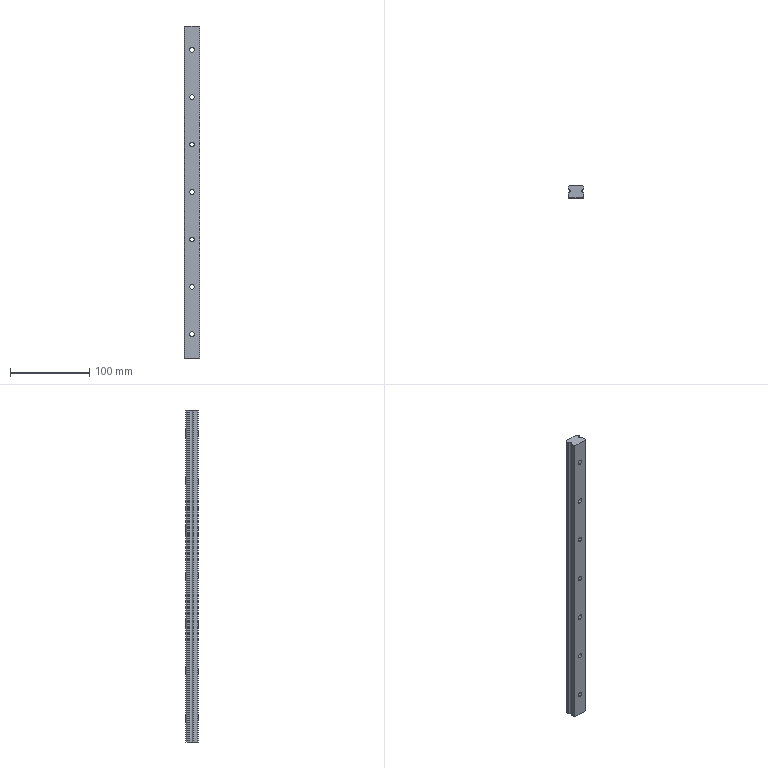Part | SolidWorks | features BaseBody 1 | 1 solid | 51 faces | box 20 x 15.5 x 420 mm | volume 115251 mm3 | cylinder 32 | plane 19 | commonest cylinder face diameters 6 x14 9.5 x14 3 x2 5 x2
STEP:
#1=CARTESIAN_POINT('',(-10.,6.18,-210.));
#2=VERTEX_POINT('',#1);
#3=CARTESIAN_POINT('',(-10.,0.6,-210.));
#4=VERTEX_POINT('',#3);
#5=CARTESIAN_POINT('',(-10.,6.18,-210.));
#6=DIRECTION('',(0.,-1.,0.));
#7=VECTOR('',#6,1000.);
#8=LINE('',#5,#7);
#9=EDGE_CURVE('',#2,#4,#8,.T.);
#10=ORIENTED_EDGE('',*,*,#9,.T.);
#11=CARTESIAN_POINT('',(-10.,0.6,210.));
#12=VERTEX_POINT('',#11);
#13=CARTESIAN_POINT('',(-10.,0.6,210.));
#14=DIRECTION('',(0.,0.,-1.));
#15=VECTOR('',#14,1000.);
#16=LINE('',#13,#15);
#17=EDGE_CURVE('',#12,#4,#16,.T.);
#18=ORIENTED_EDGE('',*,*,#17,.F.);
#19=CARTESIAN_POINT('',(-10.,6.18,210.));
#20=VERTEX_POINT('',#19);
#21=CARTESIAN_POINT('',(-10.,6.18,210.));
#22=DIRECTION('',(0.,-1.,0.));
#23=VECTOR('',#22,1000.);
#24=LINE('',#21,#23);
#25=EDGE_CURVE('',#20,#12,#24,.T.);
#26=ORIENTED_EDGE('',*,*,#25,.F.);
#27=CARTESIAN_POINT('',(-10.,6.18,210.));
#28=DIRECTION('',(0.,0.,-1.));
#29=VECTOR('',#28,1000.);
#30=LINE('',#27,#29);
#31=EDGE_CURVE('',#20,#2,#30,.T.);
#32=ORIENTED_EDGE('',*,*,#31,.T.);
#33=EDGE_LOOP('',(#10,#18,#26,#32));
#34=FACE_OUTER_BOUND('',#33,.T.);
#35=CARTESIAN_POINT('',(-10.,6.18,210.));
#36=DIRECTION('',(1.,0.,0.));
#37=DIRECTION('',(0.,0.,-1.));
#38=AXIS2_PLACEMENT_3D('',#35,#36,#37);
#39=PLANE('',#38);
#40=ADVANCED_FACE('',(#34),#39,.F.);
#41=CARTESIAN_POINT('',(-9.062,10.998,-210.));
#42=VERTEX_POINT('',#41);
#43=CARTESIAN_POINT('',(-10.,8.68,-210.));
#44=DIRECTION('',(0.,0.,1.));
#45=DIRECTION('',(1.,0.,0.));
#46=AXIS2_PLACEMENT_3D('',#43,#44,#45);
#47=CIRCLE('',#46,2.5);
#48=EDGE_CURVE('',#2,#42,#47,.T.);
#49=ORIENTED_EDGE('',*,*,#48,.F.);
#50=ORIENTED_EDGE('',*,*,#31,.F.);
#51=CARTESIAN_POINT('',(-9.062,10.998,210.));
#52=VERTEX_POINT('',#51);
#53=CARTESIAN_POINT('',(-10.,8.68,210.));
#54=DIRECTION('',(0.,0.,1.));
#55=DIRECTION('',(1.,0.,0.));
#56=AXIS2_PLACEMENT_3D('',#53,#54,#55);
#57=CIRCLE('',#56,2.5);
#58=EDGE_CURVE('',#20,#52,#57,.T.);
#59=ORIENTED_EDGE('',*,*,#58,.T.);
#60=CARTESIAN_POINT('',(-9.062,10.998,210.));
#61=DIRECTION('',(0.,0.,-1.));
#62=VECTOR('',#61,1000.);
#63=LINE('',#60,#62);
#64=EDGE_CURVE('',#52,#42,#63,.T.);
#65=ORIENTED_EDGE('',*,*,#64,.T.);
#66=EDGE_LOOP('',(#49,#50,#59,#65));
#67=FACE_OUTER_BOUND('',#66,.T.);
#68=CARTESIAN_POINT('',(-10.,8.68,210.));
#69=DIRECTION('',(0.,0.,-1.));
#70=DIRECTION('',(-0.9816,0.191,0.));
#71=AXIS2_PLACEMENT_3D('',#68,#69,#70);
#72=CYLINDRICAL_SURFACE('',#71,2.5);
#73=ADVANCED_FACE('',(#67),#72,.F.);
#74=CARTESIAN_POINT('',(-10.,12.388,-210.));
#75=VERTEX_POINT('',#74);
#76=CARTESIAN_POINT('',(-8.5,12.388,-210.));
#77=DIRECTION('',(0.,0.,1.));
#78=DIRECTION('',(1.,0.,0.));
#79=AXIS2_PLACEMENT_3D('',#76,#77,#78);
#80=CIRCLE('',#79,1.5);
#81=EDGE_CURVE('',#75,#42,#80,.T.);
#82=ORIENTED_EDGE('',*,*,#81,.T.);
#83=ORIENTED_EDGE('',*,*,#64,.F.);
#84=CARTESIAN_POINT('',(-10.,12.388,210.));
#85=VERTEX_POINT('',#84);
#86=CARTESIAN_POINT('',(-8.5,12.388,210.));
#87=DIRECTION('',(0.,0.,1.));
#88=DIRECTION('',(1.,0.,0.));
#89=AXIS2_PLACEMENT_3D('',#86,#87,#88);
#90=CIRCLE('',#89,1.5);
#91=EDGE_CURVE('',#85,#52,#90,.T.);
#92=ORIENTED_EDGE('',*,*,#91,.F.);
#93=CARTESIAN_POINT('',(-10.,12.388,210.));
#94=DIRECTION('',(0.,0.,-1.));
#95=VECTOR('',#94,1000.);
#96=LINE('',#93,#95);
#97=EDGE_CURVE('',#85,#75,#96,.T.);
#98=ORIENTED_EDGE('',*,*,#97,.T.);
#99=EDGE_LOOP('',(#82,#83,#92,#98));
#100=FACE_OUTER_BOUND('',#99,.T.);
#101=CARTESIAN_POINT('',(-8.5,12.388,210.));
#102=DIRECTION('',(0.,0.,-1.));
#103=DIRECTION('',(0.8292,0.559,0.));
#104=AXIS2_PLACEMENT_3D('',#101,#102,#103);
#105=CYLINDRICAL_SURFACE('',#104,1.5);
#106=ADVANCED_FACE('',(#100),#105,.T.);
#107=CARTESIAN_POINT('',(-10.,14.043,-210.));
#108=VERTEX_POINT('',#107);
#109=CARTESIAN_POINT('',(-10.,14.043,-210.));
#110=DIRECTION('',(0.,-1.,0.));
#111=VECTOR('',#110,1000.);
#112=LINE('',#109,#111);
#113=EDGE_CURVE('',#108,#75,#112,.T.);
#114=ORIENTED_EDGE('',*,*,#113,.T.);
#115=ORIENTED_EDGE('',*,*,#97,.F.);
#116=CARTESIAN_POINT('',(-10.,14.043,210.));
#117=VERTEX_POINT('',#116);
#118=CARTESIAN_POINT('',(-10.,14.043,210.));
#119=DIRECTION('',(0.,-1.,0.));
#120=VECTOR('',#119,1000.);
#121=LINE('',#118,#120);
#122=EDGE_CURVE('',#117,#85,#121,.T.);
#123=ORIENTED_EDGE('',*,*,#122,.F.);
#124=CARTESIAN_POINT('',(-10.,14.043,210.));
#125=DIRECTION('',(0.,0.,-1.));
#126=VECTOR('',#125,1000.);
#127=LINE('',#124,#126);
#128=EDGE_CURVE('',#117,#108,#127,.T.);
#129=ORIENTED_EDGE('',*,*,#128,.T.);
#130=EDGE_LOOP('',(#114,#115,#123,#129));
#131=FACE_OUTER_BOUND('',#130,.T.);
#132=CARTESIAN_POINT('',(-10.,14.043,210.));
#133=DIRECTION('',(1.,0.,0.));
#134=DIRECTION('',(0.,0.,-1.));
#135=AXIS2_PLACEMENT_3D('',#132,#133,#134);
#136=PLANE('',#135);
#137=ADVANCED_FACE('',(#131),#136,.F.);
#138=CARTESIAN_POINT('',(-8.543,15.5,-210.));
#139=VERTEX_POINT('',#138);
#140=CARTESIAN_POINT('',(-8.543,15.5,-210.));
#141=DIRECTION('',(-0.7071,-0.7071,0.));
#142=VECTOR('',#141,1000.);
#143=LINE('',#140,#142);
#144=EDGE_CURVE('',#139,#108,#143,.T.);
#145=ORIENTED_EDGE('',*,*,#144,.T.);
#146=ORIENTED_EDGE('',*,*,#128,.F.);
#147=CARTESIAN_POINT('',(-8.543,15.5,210.));
#148=VERTEX_POINT('',#147);
#149=CARTESIAN_POINT('',(-8.543,15.5,210.));
#150=DIRECTION('',(-0.7071,-0.7071,0.));
#151=VECTOR('',#150,1000.);
#152=LINE('',#149,#151);
#153=EDGE_CURVE('',#148,#117,#152,.T.);
#154=ORIENTED_EDGE('',*,*,#153,.F.);
#155=CARTESIAN_POINT('',(-8.543,15.5,210.));
#156=DIRECTION('',(0.,0.,-1.));
#157=VECTOR('',#156,1000.);
#158=LINE('',#155,#157);
#159=EDGE_CURVE('',#148,#139,#158,.T.);
#160=ORIENTED_EDGE('',*,*,#159,.T.);
#161=EDGE_LOOP('',(#145,#146,#154,#160));
#162=FACE_OUTER_BOUND('',#161,.T.);
#163=CARTESIAN_POINT('',(-8.543,15.5,210.));
#164=DIRECTION('',(0.7071,-0.7071,0.));
#165=DIRECTION('',(0.7071,0.7071,0.));
#166=AXIS2_PLACEMENT_3D('',#163,#164,#165);
#167=PLANE('',#166);
#168=ADVANCED_FACE('',(#162),#167,.F.);
#169=CARTESIAN_POINT('',(0.,15.5,-124.75));
#170=VERTEX_POINT('',#169);
#171=CARTESIAN_POINT('',(0.,15.5,-115.25));
#172=VERTEX_POINT('',#171);
#173=CARTESIAN_POINT('',(0.,15.5,-120.));
#174=DIRECTION('',(0.,-1.,0.));
#175=DIRECTION('',(0.,0.,-1.));
#176=AXIS2_PLACEMENT_3D('',#173,#174,#175);
#177=CIRCLE('',#176,4.75);
#178=EDGE_CURVE('',#170,#172,#177,.T.);
#179=ORIENTED_EDGE('',*,*,#178,.T.);
#180=CARTESIAN_POINT('',(0.,15.5,-120.));
#181=DIRECTION('',(0.,-1.,0.));
#182=DIRECTION('',(0.,0.,-1.));
#183=AXIS2_PLACEMENT_3D('',#180,#181,#182);
#184=CIRCLE('',#183,4.75);
#185=EDGE_CURVE('',#172,#170,#184,.T.);
#186=ORIENTED_EDGE('',*,*,#185,.T.);
#187=EDGE_LOOP('',(#179,#186));
#188=FACE_BOUND('',#187,.T.);
#189=CARTESIAN_POINT('',(0.,15.5,-64.75));
#190=VERTEX_POINT('',#189);
#191=CARTESIAN_POINT('',(0.,15.5,-55.25));
#192=VERTEX_POINT('',#191);
#193=CARTESIAN_POINT('',(0.,15.5,-60.));
#194=DIRECTION('',(0.,-1.,0.));
#195=DIRECTION('',(0.,0.,-1.));
#196=AXIS2_PLACEMENT_3D('',#193,#194,#195);
#197=CIRCLE('',#196,4.75);
#198=EDGE_CURVE('',#190,#192,#197,.T.);
#199=ORIENTED_EDGE('',*,*,#198,.T.);
#200=CARTESIAN_POINT('',(0.,15.5,-60.));
#201=DIRECTION('',(0.,-1.,0.));
#202=DIRECTION('',(0.,0.,-1.));
#203=AXIS2_PLACEMENT_3D('',#200,#201,#202);
#204=CIRCLE('',#203,4.75);
#205=EDGE_CURVE('',#192,#190,#204,.T.);
#206=ORIENTED_EDGE('',*,*,#205,.T.);
#207=EDGE_LOOP('',(#199,#206));
#208=FACE_BOUND('',#207,.T.);
#209=CARTESIAN_POINT('',(0.,15.5,-4.75));
#210=VERTEX_POINT('',#209);
#211=CARTESIAN_POINT('',(0.,15.5,4.75));
#212=VERTEX_POINT('',#211);
#213=CARTESIAN_POINT('',(0.,15.5,0.));
#214=DIRECTION('',(0.,-1.,0.));
#215=DIRECTION('',(0.,0.,-1.));
#216=AXIS2_PLACEMENT_3D('',#213,#214,#215);
#217=CIRCLE('',#216,4.75);
#218=EDGE_CURVE('',#210,#212,#217,.T.);
#219=ORIENTED_EDGE('',*,*,#218,.T.);
#220=CARTESIAN_POINT('',(0.,15.5,0.));
#221=DIRECTION('',(0.,-1.,0.));
#222=DIRECTION('',(0.,0.,-1.));
#223=AXIS2_PLACEMENT_3D('',#220,#221,#222);
#224=CIRCLE('',#223,4.75);
#225=EDGE_CURVE('',#212,#210,#224,.T.);
#226=ORIENTED_EDGE('',*,*,#225,.T.);
#227=EDGE_LOOP('',(#219,#226));
#228=FACE_BOUND('',#227,.T.);
#229=CARTESIAN_POINT('',(0.,15.5,55.25));
#230=VERTEX_POINT('',#229);
#231=CARTESIAN_POINT('',(0.,15.5,64.75));
#232=VERTEX_POINT('',#231);
#233=CARTESIAN_POINT('',(0.,15.5,60.));
#234=DIRECTION('',(0.,-1.,0.));
#235=DIRECTION('',(0.,0.,-1.));
#236=AXIS2_PLACEMENT_3D('',#233,#234,#235);
#237=CIRCLE('',#236,4.75);
#238=EDGE_CURVE('',#230,#232,#237,.T.);
#239=ORIENTED_EDGE('',*,*,#238,.T.);
#240=CARTESIAN_POINT('',(0.,15.5,60.));
#241=DIRECTION('',(0.,-1.,0.));
#242=DIRECTION('',(0.,0.,-1.));
#243=AXIS2_PLACEMENT_3D('',#240,#241,#242);
#244=CIRCLE('',#243,4.75);
#245=EDGE_CURVE('',#232,#230,#244,.T.);
#246=ORIENTED_EDGE('',*,*,#245,.T.);
#247=EDGE_LOOP('',(#239,#246));
#248=FACE_BOUND('',#247,.T.);
#249=CARTESIAN_POINT('',(0.,15.5,115.25));
#250=VERTEX_POINT('',#249);
#251=CARTESIAN_POINT('',(0.,15.5,124.75));
#252=VERTEX_POINT('',#251);
#253=CARTESIAN_POINT('',(0.,15.5,120.));
#254=DIRECTION('',(0.,-1.,0.));
#255=DIRECTION('',(0.,0.,-1.));
#256=AXIS2_PLACEMENT_3D('',#253,#254,#255);
#257=CIRCLE('',#256,4.75);
#258=EDGE_CURVE('',#250,#252,#257,.T.);
#259=ORIENTED_EDGE('',*,*,#258,.T.);
#260=CARTESIAN_POINT('',(0.,15.5,120.));
#261=DIRECTION('',(0.,-1.,0.));
#262=DIRECTION('',(0.,0.,-1.));
#263=AXIS2_PLACEMENT_3D('',#260,#261,#262);
#264=CIRCLE('',#263,4.75);
#265=EDGE_CURVE('',#252,#250,#264,.T.);
#266=ORIENTED_EDGE('',*,*,#265,.T.);
#267=EDGE_LOOP('',(#259,#266));
#268=FACE_BOUND('',#267,.T.);
#269=CARTESIAN_POINT('',(0.,15.5,175.25));
#270=VERTEX_POINT('',#269);
#271=CARTESIAN_POINT('',(0.,15.5,184.75));
#272=VERTEX_POINT('',#271);
#273=CARTESIAN_POINT('',(0.,15.5,180.));
#274=DIRECTION('',(0.,-1.,0.));
#275=DIRECTION('',(0.,0.,-1.));
#276=AXIS2_PLACEMENT_3D('',#273,#274,#275);
#277=CIRCLE('',#276,4.75);
#278=EDGE_CURVE('',#270,#272,#277,.T.);
#279=ORIENTED_EDGE('',*,*,#278,.T.);
#280=CARTESIAN_POINT('',(0.,15.5,180.));
#281=DIRECTION('',(0.,-1.,0.));
#282=DIRECTION('',(0.,0.,-1.));
#283=AXIS2_PLACEMENT_3D('',#280,#281,#282);
#284=CIRCLE('',#283,4.75);
#285=EDGE_CURVE('',#272,#270,#284,.T.);
#286=ORIENTED_EDGE('',*,*,#285,.T.);
#287=EDGE_LOOP('',(#279,#286));
#288=FACE_BOUND('',#287,.T.);
#289=CARTESIAN_POINT('',(0.,15.5,-184.75));
#290=VERTEX_POINT('',#289);
#291=CARTESIAN_POINT('',(0.,15.5,-175.25));
#292=VERTEX_POINT('',#291);
#293=CARTESIAN_POINT('',(0.,15.5,-180.));
#294=DIRECTION('',(0.,-1.,0.));
#295=DIRECTION('',(0.,0.,-1.));
#296=AXIS2_PLACEMENT_3D('',#293,#294,#295);
#297=CIRCLE('',#296,4.75);
#298=EDGE_CURVE('',#290,#292,#297,.T.);
#299=ORIENTED_EDGE('',*,*,#298,.T.);
#300=CARTESIAN_POINT('',(0.,15.5,-180.));
#301=DIRECTION('',(0.,-1.,0.));
#302=DIRECTION('',(0.,0.,-1.));
#303=AXIS2_PLACEMENT_3D('',#300,#301,#302);
#304=CIRCLE('',#303,4.75);
#305=EDGE_CURVE('',#292,#290,#304,.T.);
#306=ORIENTED_EDGE('',*,*,#305,.T.);
#307=EDGE_LOOP('',(#299,#306));
#308=FACE_BOUND('',#307,.T.);
#309=CARTESIAN_POINT('',(8.543,15.5,-210.));
#310=VERTEX_POINT('',#309);
#311=CARTESIAN_POINT('',(8.543,15.5,-210.));
#312=DIRECTION('',(-1.,0.,0.));
#313=VECTOR('',#312,1000.);
#314=LINE('',#311,#313);
#315=EDGE_CURVE('',#310,#139,#314,.T.);
#316=ORIENTED_EDGE('',*,*,#315,.T.);
#317=ORIENTED_EDGE('',*,*,#159,.F.);
#318=CARTESIAN_POINT('',(8.543,15.5,210.));
#319=VERTEX_POINT('',#318);
#320=CARTESIAN_POINT('',(8.543,15.5,210.));
#321=DIRECTION('',(-1.,0.,0.));
#322=VECTOR('',#321,1000.);
#323=LINE('',#320,#322);
#324=EDGE_CURVE('',#319,#148,#323,.T.);
#325=ORIENTED_EDGE('',*,*,#324,.F.);
#326=CARTESIAN_POINT('',(8.543,15.5,210.));
#327=DIRECTION('',(0.,0.,-1.));
#328=VECTOR('',#327,1000.);
#329=LINE('',#326,#328);
#330=EDGE_CURVE('',#319,#310,#329,.T.);
#331=ORIENTED_EDGE('',*,*,#330,.T.);
#332=EDGE_LOOP('',(#316,#317,#325,#331));
#333=FACE_OUTER_BOUND('',#332,.T.);
#334=CARTESIAN_POINT('',(8.543,15.5,210.));
#335=DIRECTION('',(0.,-1.,0.));
#336=DIRECTION('',(0.,0.,-1.));
#337=AXIS2_PLACEMENT_3D('',#334,#335,#336);
#338=PLANE('',#337);
#339=ADVANCED_FACE('',(#188,#208,#228,#248,#268,#288,#308,#333),#338,.F.);
#340=CARTESIAN_POINT('',(10.,14.043,-210.));
#341=VERTEX_POINT('',#340);
#342=CARTESIAN_POINT('',(10.,14.043,-210.));
#343=DIRECTION('',(-0.7071,0.7071,0.));
#344=VECTOR('',#343,1000.);
#345=LINE('',#342,#344);
#346=EDGE_CURVE('',#341,#310,#345,.T.);
#347=ORIENTED_EDGE('',*,*,#346,.T.);
#348=ORIENTED_EDGE('',*,*,#330,.F.);
#349=CARTESIAN_POINT('',(10.,14.043,210.));
#350=VERTEX_POINT('',#349);
#351=CARTESIAN_POINT('',(10.,14.043,210.));
#352=DIRECTION('',(-0.7071,0.7071,0.));
#353=VECTOR('',#352,1000.);
#354=LINE('',#351,#353);
#355=EDGE_CURVE('',#350,#319,#354,.T.);
#356=ORIENTED_EDGE('',*,*,#355,.F.);
#357=CARTESIAN_POINT('',(10.,14.043,210.));
#358=DIRECTION('',(0.,0.,-1.));
#359=VECTOR('',#358,1000.);
#360=LINE('',#357,#359);
#361=EDGE_CURVE('',#350,#341,#360,.T.);
#362=ORIENTED_EDGE('',*,*,#361,.T.);
#363=EDGE_LOOP('',(#347,#348,#356,#362));
#364=FACE_OUTER_BOUND('',#363,.T.);
#365=CARTESIAN_POINT('',(10.,14.043,210.));
#366=DIRECTION('',(-0.7071,-0.7071,0.));
#367=DIRECTION('',(0.7071,-0.7071,0.));
#368=AXIS2_PLACEMENT_3D('',#365,#366,#367);
#369=PLANE('',#368);
#370=ADVANCED_FACE('',(#364),#369,.F.);
#371=CARTESIAN_POINT('',(10.,12.388,-210.));
#372=VERTEX_POINT('',#371);
#373=CARTESIAN_POINT('',(10.,12.388,-210.));
#374=DIRECTION('',(0.,1.,0.));
#375=VECTOR('',#374,1000.);
#376=LINE('',#373,#375);
#377=EDGE_CURVE('',#372,#341,#376,.T.);
#378=ORIENTED_EDGE('',*,*,#377,.T.);
#379=ORIENTED_EDGE('',*,*,#361,.F.);
#380=CARTESIAN_POINT('',(10.,12.388,210.));
#381=VERTEX_POINT('',#380);
#382=CARTESIAN_POINT('',(10.,12.388,210.));
#383=DIRECTION('',(0.,1.,0.));
#384=VECTOR('',#383,1000.);
#385=LINE('',#382,#384);
#386=EDGE_CURVE('',#381,#350,#385,.T.);
#387=ORIENTED_EDGE('',*,*,#386,.F.);
#388=CARTESIAN_POINT('',(10.,12.388,210.));
#389=DIRECTION('',(0.,0.,-1.));
#390=VECTOR('',#389,1000.);
#391=LINE('',#388,#390);
#392=EDGE_CURVE('',#381,#372,#391,.T.);
#393=ORIENTED_EDGE('',*,*,#392,.T.);
#394=EDGE_LOOP('',(#378,#379,#387,#393));
#395=FACE_OUTER_BOUND('',#394,.T.);
#396=CARTESIAN_POINT('',(10.,12.388,210.));
#397=DIRECTION('',(-1.,0.,0.));
#398=DIRECTION('',(0.,0.,1.));
#399=AXIS2_PLACEMENT_3D('',#396,#397,#398);
#400=PLANE('',#399);
#401=ADVANCED_FACE('',(#395),#400,.F.);
#402=CARTESIAN_POINT('',(9.062,10.998,-210.));
#403=VERTEX_POINT('',#402);
#404=CARTESIAN_POINT('',(8.5,12.388,-210.));
#405=DIRECTION('',(0.,0.,1.));
#406=DIRECTION('',(1.,0.,0.));
#407=AXIS2_PLACEMENT_3D('',#404,#405,#406);
#408=CIRCLE('',#407,1.5);
#409=EDGE_CURVE('',#403,#372,#408,.T.);
#410=ORIENTED_EDGE('',*,*,#409,.T.);
#411=ORIENTED_EDGE('',*,*,#392,.F.);
#412=CARTESIAN_POINT('',(9.062,10.998,210.));
#413=VERTEX_POINT('',#412);
#414=CARTESIAN_POINT('',(8.5,12.388,210.));
#415=DIRECTION('',(0.,0.,1.));
#416=DIRECTION('',(1.,0.,0.));
#417=AXIS2_PLACEMENT_3D('',#414,#415,#416);
#418=CIRCLE('',#417,1.5);
#419=EDGE_CURVE('',#413,#381,#418,.T.);
#420=ORIENTED_EDGE('',*,*,#419,.F.);
#421=CARTESIAN_POINT('',(9.062,10.998,210.));
#422=DIRECTION('',(0.,0.,-1.));
#423=VECTOR('',#422,1000.);
#424=LINE('',#421,#423);
#425=EDGE_CURVE('',#413,#403,#424,.T.);
#426=ORIENTED_EDGE('',*,*,#425,.T.);
#427=EDGE_LOOP('',(#410,#411,#420,#426));
#428=FACE_OUTER_BOUND('',#427,.T.);
#429=CARTESIAN_POINT('',(8.5,12.388,210.));
#430=DIRECTION('',(0.,0.,-1.));
#431=DIRECTION('',(-0.8292,0.559,0.));
#432=AXIS2_PLACEMENT_3D('',#429,#430,#431);
#433=CYLINDRICAL_SURFACE('',#432,1.5);
#434=ADVANCED_FACE('',(#428),#433,.T.);
#435=CARTESIAN_POINT('',(10.,6.18,-210.));
#436=VERTEX_POINT('',#435);
#437=CARTESIAN_POINT('',(10.,8.68,-210.));
#438=DIRECTION('',(0.,0.,1.));
#439=DIRECTION('',(1.,0.,0.));
#440=AXIS2_PLACEMENT_3D('',#437,#438,#439);
#441=CIRCLE('',#440,2.5);
#442=EDGE_CURVE('',#403,#436,#441,.T.);
#443=ORIENTED_EDGE('',*,*,#442,.F.);
#444=ORIENTED_EDGE('',*,*,#425,.F.);
#445=CARTESIAN_POINT('',(10.,6.18,210.));
#446=VERTEX_POINT('',#445);
#447=CARTESIAN_POINT('',(10.,8.68,210.));
#448=DIRECTION('',(0.,0.,1.));
#449=DIRECTION('',(1.,0.,0.));
#450=AXIS2_PLACEMENT_3D('',#447,#448,#449);
#451=CIRCLE('',#450,2.5);
#452=EDGE_CURVE('',#413,#446,#451,.T.);
#453=ORIENTED_EDGE('',*,*,#452,.T.);
#454=CARTESIAN_POINT('',(10.,6.18,210.));
#455=DIRECTION('',(0.,0.,-1.));
#456=VECTOR('',#455,1000.);
#457=LINE('',#454,#456);
#458=EDGE_CURVE('',#446,#436,#457,.T.);
#459=ORIENTED_EDGE('',*,*,#458,.T.);
#460=EDGE_LOOP('',(#443,#444,#453,#459));
#461=FACE_OUTER_BOUND('',#460,.T.);
#462=CARTESIAN_POINT('',(10.,8.68,210.));
#463=DIRECTION('',(0.,0.,-1.));
#464=DIRECTION('',(0.9816,0.191,0.));
#465=AXIS2_PLACEMENT_3D('',#462,#463,#464);
#466=CYLINDRICAL_SURFACE('',#465,2.5);
#467=ADVANCED_FACE('',(#461),#466,.F.);
#468=CARTESIAN_POINT('',(10.,0.6,-210.));
#469=VERTEX_POINT('',#468);
#470=CARTESIAN_POINT('',(10.,0.6,-210.));
#471=DIRECTION('',(0.,1.,0.));
#472=VECTOR('',#471,1000.);
#473=LINE('',#470,#472);
#474=EDGE_CURVE('',#469,#436,#473,.T.);
#475=ORIENTED_EDGE('',*,*,#474,.T.);
#476=ORIENTED_EDGE('',*,*,#458,.F.);
#477=CARTESIAN_POINT('',(10.,0.6,210.));
#478=VERTEX_POINT('',#477);
#479=CARTESIAN_POINT('',(10.,0.6,210.));
#480=DIRECTION('',(0.,1.,0.));
#481=VECTOR('',#480,1000.);
#482=LINE('',#479,#481);
#483=EDGE_CURVE('',#478,#446,#482,.T.);
#484=ORIENTED_EDGE('',*,*,#483,.F.);
#485=CARTESIAN_POINT('',(10.,0.6,210.));
#486=DIRECTION('',(0.,0.,-1.));
#487=VECTOR('',#486,1000.);
#488=LINE('',#485,#487);
#489=EDGE_CURVE('',#478,#469,#488,.T.);
#490=ORIENTED_EDGE('',*,*,#489,.T.);
#491=EDGE_LOOP('',(#475,#476,#484,#490));
#492=FACE_OUTER_BOUND('',#491,.T.);
#493=CARTESIAN_POINT('',(10.,0.6,210.));
#494=DIRECTION('',(-1.,0.,0.));
#495=DIRECTION('',(0.,0.,1.));
#496=AXIS2_PLACEMENT_3D('',#493,#494,#495);
#497=PLANE('',#496);
#498=ADVANCED_FACE('',(#492),#497,.F.);
#499=CARTESIAN_POINT('',(9.4,0.,-210.));
#500=VERTEX_POINT('',#499);
#501=CARTESIAN_POINT('',(9.4,0.,-210.));
#502=DIRECTION('',(0.7071,0.7071,0.));
#503=VECTOR('',#502,1000.);
#504=LINE('',#501,#503);
#505=EDGE_CURVE('',#500,#469,#504,.T.);
#506=ORIENTED_EDGE('',*,*,#505,.T.);
#507=ORIENTED_EDGE('',*,*,#489,.F.);
#508=CARTESIAN_POINT('',(9.4,0.,210.));
#509=VERTEX_POINT('',#508);
#510=CARTESIAN_POINT('',(9.4,0.,210.));
#511=DIRECTION('',(0.7071,0.7071,0.));
#512=VECTOR('',#511,1000.);
#513=LINE('',#510,#512);
#514=EDGE_CURVE('',#509,#478,#513,.T.);
#515=ORIENTED_EDGE('',*,*,#514,.F.);
#516=CARTESIAN_POINT('',(9.4,0.,210.));
#517=DIRECTION('',(0.,0.,-1.));
#518=VECTOR('',#517,1000.);
#519=LINE('',#516,#518);
#520=EDGE_CURVE('',#509,#500,#519,.T.);
#521=ORIENTED_EDGE('',*,*,#520,.T.);
#522=EDGE_LOOP('',(#506,#507,#515,#521));
#523=FACE_OUTER_BOUND('',#522,.T.);
#524=CARTESIAN_POINT('',(9.4,0.,210.));
#525=DIRECTION('',(-0.7071,0.7071,0.));
#526=DIRECTION('',(-0.7071,-0.7071,0.));
#527=AXIS2_PLACEMENT_3D('',#524,#525,#526);
#528=PLANE('',#527);
#529=ADVANCED_FACE('',(#523),#528,.F.);
#530=CARTESIAN_POINT('',(0.,0.,-117.));
#531=VERTEX_POINT('',#530);
#532=CARTESIAN_POINT('',(0.,0.,-123.));
#533=VERTEX_POINT('',#532);
#534=CARTESIAN_POINT('',(0.,0.,-120.));
#535=DIRECTION('',(0.,-1.,0.));
#536=DIRECTION('',(0.,0.,-1.));
#537=AXIS2_PLACEMENT_3D('',#534,#535,#536);
#538=CIRCLE('',#537,3.);
#539=EDGE_CURVE('',#531,#533,#538,.T.);
#540=ORIENTED_EDGE('',*,*,#539,.F.);
#541=CARTESIAN_POINT('',(0.,0.,-120.));
#542=DIRECTION('',(0.,-1.,0.));
#543=DIRECTION('',(0.,0.,-1.));
#544=AXIS2_PLACEMENT_3D('',#541,#542,#543);
#545=CIRCLE('',#544,3.);
#546=EDGE_CURVE('',#533,#531,#545,.T.);
#547=ORIENTED_EDGE('',*,*,#546,.F.);
#548=EDGE_LOOP('',(#540,#547));
#549=FACE_BOUND('',#548,.T.);
#550=CARTESIAN_POINT('',(0.,0.,-57.));
#551=VERTEX_POINT('',#550);
#552=CARTESIAN_POINT('',(0.,0.,-63.));
#553=VERTEX_POINT('',#552);
#554=CARTESIAN_POINT('',(0.,0.,-60.));
#555=DIRECTION('',(0.,-1.,0.));
#556=DIRECTION('',(0.,0.,-1.));
#557=AXIS2_PLACEMENT_3D('',#554,#555,#556);
#558=CIRCLE('',#557,3.);
#559=EDGE_CURVE('',#551,#553,#558,.T.);
#560=ORIENTED_EDGE('',*,*,#559,.F.);
#561=CARTESIAN_POINT('',(0.,0.,-60.));
#562=DIRECTION('',(0.,-1.,0.));
#563=DIRECTION('',(0.,0.,-1.));
#564=AXIS2_PLACEMENT_3D('',#561,#562,#563);
#565=CIRCLE('',#564,3.);
#566=EDGE_CURVE('',#553,#551,#565,.T.);
#567=ORIENTED_EDGE('',*,*,#566,.F.);
#568=EDGE_LOOP('',(#560,#567));
#569=FACE_BOUND('',#568,.T.);
#570=CARTESIAN_POINT('',(0.,0.,3.));
#571=VERTEX_POINT('',#570);
#572=CARTESIAN_POINT('',(0.,0.,-3.));
#573=VERTEX_POINT('',#572);
#574=CARTESIAN_POINT('',(0.,0.,0.));
#575=DIRECTION('',(0.,-1.,0.));
#576=DIRECTION('',(0.,0.,-1.));
#577=AXIS2_PLACEMENT_3D('',#574,#575,#576);
#578=CIRCLE('',#577,3.);
#579=EDGE_CURVE('',#571,#573,#578,.T.);
#580=ORIENTED_EDGE('',*,*,#579,.F.);
#581=CARTESIAN_POINT('',(0.,0.,0.));
#582=DIRECTION('',(0.,-1.,0.));
#583=DIRECTION('',(0.,0.,-1.));
#584=AXIS2_PLACEMENT_3D('',#581,#582,#583);
#585=CIRCLE('',#584,3.);
#586=EDGE_CURVE('',#573,#571,#585,.T.);
#587=ORIENTED_EDGE('',*,*,#586,.F.);
#588=EDGE_LOOP('',(#580,#587));
#589=FACE_BOUND('',#588,.T.);
#590=CARTESIAN_POINT('',(0.,0.,63.));
#591=VERTEX_POINT('',#590);
#592=CARTESIAN_POINT('',(0.,0.,57.));
#593=VERTEX_POINT('',#592);
#594=CARTESIAN_POINT('',(0.,0.,60.));
#595=DIRECTION('',(0.,-1.,0.));
#596=DIRECTION('',(0.,0.,-1.));
#597=AXIS2_PLACEMENT_3D('',#594,#595,#596);
#598=CIRCLE('',#597,3.);
#599=EDGE_CURVE('',#591,#593,#598,.T.);
#600=ORIENTED_EDGE('',*,*,#599,.F.);
#601=CARTESIAN_POINT('',(0.,0.,60.));
#602=DIRECTION('',(0.,-1.,0.));
#603=DIRECTION('',(0.,0.,-1.));
#604=AXIS2_PLACEMENT_3D('',#601,#602,#603);
#605=CIRCLE('',#604,3.);
#606=EDGE_CURVE('',#593,#591,#605,.T.);
#607=ORIENTED_EDGE('',*,*,#606,.F.);
#608=EDGE_LOOP('',(#600,#607));
#609=FACE_BOUND('',#608,.T.);
#610=CARTESIAN_POINT('',(0.,0.,123.));
#611=VERTEX_POINT('',#610);
#612=CARTESIAN_POINT('',(0.,0.,117.));
#613=VERTEX_POINT('',#612);
#614=CARTESIAN_POINT('',(0.,0.,120.));
#615=DIRECTION('',(0.,-1.,0.));
#616=DIRECTION('',(0.,0.,-1.));
#617=AXIS2_PLACEMENT_3D('',#614,#615,#616);
#618=CIRCLE('',#617,3.);
#619=EDGE_CURVE('',#611,#613,#618,.T.);
#620=ORIENTED_EDGE('',*,*,#619,.F.);
#621=CARTESIAN_POINT('',(0.,0.,120.));
#622=DIRECTION('',(0.,-1.,0.));
#623=DIRECTION('',(0.,0.,-1.));
#624=AXIS2_PLACEMENT_3D('',#621,#622,#623);
#625=CIRCLE('',#624,3.);
#626=EDGE_CURVE('',#613,#611,#625,.T.);
#627=ORIENTED_EDGE('',*,*,#626,.F.);
#628=EDGE_LOOP('',(#620,#627));
#629=FACE_BOUND('',#628,.T.);
#630=CARTESIAN_POINT('',(0.,0.,183.));
#631=VERTEX_POINT('',#630);
#632=CARTESIAN_POINT('',(0.,0.,177.));
#633=VERTEX_POINT('',#632);
#634=CARTESIAN_POINT('',(0.,0.,180.));
#635=DIRECTION('',(0.,-1.,0.));
#636=DIRECTION('',(0.,0.,-1.));
#637=AXIS2_PLACEMENT_3D('',#634,#635,#636);
#638=CIRCLE('',#637,3.);
#639=EDGE_CURVE('',#631,#633,#638,.T.);
#640=ORIENTED_EDGE('',*,*,#639,.F.);
#641=CARTESIAN_POINT('',(0.,0.,180.));
#642=DIRECTION('',(0.,-1.,0.));
#643=DIRECTION('',(0.,0.,-1.));
#644=AXIS2_PLACEMENT_3D('',#641,#642,#643);
#645=CIRCLE('',#644,3.);
#646=EDGE_CURVE('',#633,#631,#645,.T.);
#647=ORIENTED_EDGE('',*,*,#646,.F.);
#648=EDGE_LOOP('',(#640,#647));
#649=FACE_BOUND('',#648,.T.);
#650=CARTESIAN_POINT('',(0.,0.,-177.));
#651=VERTEX_POINT('',#650);
#652=CARTESIAN_POINT('',(0.,0.,-183.));
#653=VERTEX_POINT('',#652);
#654=CARTESIAN_POINT('',(0.,0.,-180.));
#655=DIRECTION('',(0.,-1.,0.));
#656=DIRECTION('',(0.,0.,-1.));
#657=AXIS2_PLACEMENT_3D('',#654,#655,#656);
#658=CIRCLE('',#657,3.);
#659=EDGE_CURVE('',#651,#653,#658,.T.);
#660=ORIENTED_EDGE('',*,*,#659,.F.);
#661=CARTESIAN_POINT('',(0.,0.,-180.));
#662=DIRECTION('',(0.,-1.,0.));
#663=DIRECTION('',(0.,0.,-1.));
#664=AXIS2_PLACEMENT_3D('',#661,#662,#663);
#665=CIRCLE('',#664,3.);
#666=EDGE_CURVE('',#653,#651,#665,.T.);
#667=ORIENTED_EDGE('',*,*,#666,.F.);
#668=EDGE_LOOP('',(#660,#667));
#669=FACE_BOUND('',#668,.T.);
#670=CARTESIAN_POINT('',(-9.4,0.,-210.));
#671=VERTEX_POINT('',#670);
#672=CARTESIAN_POINT('',(-9.4,0.,-210.));
#673=DIRECTION('',(1.,0.,0.));
#674=VECTOR('',#673,1000.);
#675=LINE('',#672,#674);
#676=EDGE_CURVE('',#671,#500,#675,.T.);
#677=ORIENTED_EDGE('',*,*,#676,.T.);
#678=ORIENTED_EDGE('',*,*,#520,.F.);
#679=CARTESIAN_POINT('',(-9.4,0.,210.));
#680=VERTEX_POINT('',#679);
#681=CARTESIAN_POINT('',(-9.4,0.,210.));
#682=DIRECTION('',(1.,0.,0.));
#683=VECTOR('',#682,1000.);
#684=LINE('',#681,#683);
#685=EDGE_CURVE('',#680,#509,#684,.T.);
#686=ORIENTED_EDGE('',*,*,#685,.F.);
#687=CARTESIAN_POINT('',(-9.4,0.,210.));
#688=DIRECTION('',(0.,0.,-1.));
#689=VECTOR('',#688,1000.);
#690=LINE('',#687,#689);
#691=EDGE_CURVE('',#680,#671,#690,.T.);
#692=ORIENTED_EDGE('',*,*,#691,.T.);
#693=EDGE_LOOP('',(#677,#678,#686,#692));
#694=FACE_OUTER_BOUND('',#693,.T.);
#695=CARTESIAN_POINT('',(-9.4,0.,210.));
#696=DIRECTION('',(0.,1.,0.));
#697=DIRECTION('',(0.,0.,1.));
#698=AXIS2_PLACEMENT_3D('',#695,#696,#697);
#699=PLANE('',#698);
#700=ADVANCED_FACE('',(#549,#569,#589,#609,#629,#649,#669,#694),#699,.F.);
#701=CARTESIAN_POINT('',(-10.,0.6,-210.));
#702=DIRECTION('',(0.7071,-0.7071,0.));
#703=VECTOR('',#702,1000.);
#704=LINE('',#701,#703);
#705=EDGE_CURVE('',#4,#671,#704,.T.);
#706=ORIENTED_EDGE('',*,*,#705,.T.);
#707=ORIENTED_EDGE('',*,*,#691,.F.);
#708=CARTESIAN_POINT('',(-10.,0.6,210.));
#709=DIRECTION('',(0.7071,-0.7071,0.));
#710=VECTOR('',#709,1000.);
#711=LINE('',#708,#710);
#712=EDGE_CURVE('',#12,#680,#711,.T.);
#713=ORIENTED_EDGE('',*,*,#712,.F.);
#714=ORIENTED_EDGE('',*,*,#17,.T.);
#715=EDGE_LOOP('',(#706,#707,#713,#714));
#716=FACE_OUTER_BOUND('',#715,.T.);
#717=CARTESIAN_POINT('',(-10.,0.6,210.));
#718=DIRECTION('',(0.7071,0.7071,0.));
#719=DIRECTION('',(-0.7071,0.7071,0.));
#720=AXIS2_PLACEMENT_3D('',#717,#718,#719);
#721=PLANE('',#720);
#722=ADVANCED_FACE('',(#716),#721,.F.);
#723=ORIENTED_EDGE('',*,*,#25,.T.);
#724=ORIENTED_EDGE('',*,*,#712,.T.);
#725=ORIENTED_EDGE('',*,*,#685,.T.);
#726=ORIENTED_EDGE('',*,*,#514,.T.);
#727=ORIENTED_EDGE('',*,*,#483,.T.);
#728=ORIENTED_EDGE('',*,*,#452,.F.);
#729=ORIENTED_EDGE('',*,*,#419,.T.);
#730=ORIENTED_EDGE('',*,*,#386,.T.);
#731=ORIENTED_EDGE('',*,*,#355,.T.);
#732=ORIENTED_EDGE('',*,*,#324,.T.);
#733=ORIENTED_EDGE('',*,*,#153,.T.);
#734=ORIENTED_EDGE('',*,*,#122,.T.);
#735=ORIENTED_EDGE('',*,*,#91,.T.);
#736=ORIENTED_EDGE('',*,*,#58,.F.);
#737=EDGE_LOOP('',(#723,#724,#725,#726,#727,#728,#729,#730,#731,#732,#733,#734,#735,#736));
#738=FACE_OUTER_BOUND('',#737,.T.);
#739=CARTESIAN_POINT('',(10.,8.68,210.));
#740=DIRECTION('',(0.,0.,1.));
#741=DIRECTION('',(1.,0.,0.));
#742=AXIS2_PLACEMENT_3D('',#739,#740,#741);
#743=PLANE('',#742);
#744=ADVANCED_FACE('',(#738),#743,.T.);
#745=ORIENTED_EDGE('',*,*,#9,.F.);
#746=ORIENTED_EDGE('',*,*,#48,.T.);
#747=ORIENTED_EDGE('',*,*,#81,.F.);
#748=ORIENTED_EDGE('',*,*,#113,.F.);
#749=ORIENTED_EDGE('',*,*,#144,.F.);
#750=ORIENTED_EDGE('',*,*,#315,.F.);
#751=ORIENTED_EDGE('',*,*,#346,.F.);
#752=ORIENTED_EDGE('',*,*,#377,.F.);
#753=ORIENTED_EDGE('',*,*,#409,.F.);
#754=ORIENTED_EDGE('',*,*,#442,.T.);
#755=ORIENTED_EDGE('',*,*,#474,.F.);
#756=ORIENTED_EDGE('',*,*,#505,.F.);
#757=ORIENTED_EDGE('',*,*,#676,.F.);
#758=ORIENTED_EDGE('',*,*,#705,.F.);
#759=EDGE_LOOP('',(#745,#746,#747,#748,#749,#750,#751,#752,#753,#754,#755,#756,#757,#758));
#760=FACE_OUTER_BOUND('',#759,.T.);
#761=CARTESIAN_POINT('',(10.,8.68,-210.));
#762=DIRECTION('',(0.,0.,1.));
#763=DIRECTION('',(1.,0.,0.));
#764=AXIS2_PLACEMENT_3D('',#761,#762,#763);
#765=PLANE('',#764);
#766=ADVANCED_FACE('',(#760),#765,.F.);
#767=CARTESIAN_POINT('',(0.,7.5,-177.));
#768=VERTEX_POINT('',#767);
#769=CARTESIAN_POINT('',(0.,7.5,-177.));
#770=DIRECTION('',(0.,-1.,0.));
#771=VECTOR('',#770,1000.);
#772=LINE('',#769,#771);
#773=EDGE_CURVE('',#768,#651,#772,.T.);
#774=ORIENTED_EDGE('',*,*,#773,.F.);
#775=CARTESIAN_POINT('',(0.,7.5,-183.));
#776=VERTEX_POINT('',#775);
#777=CARTESIAN_POINT('',(0.,7.5,-180.));
#778=DIRECTION('',(0.,-1.,0.));
#779=DIRECTION('',(0.,0.,-1.));
#780=AXIS2_PLACEMENT_3D('',#777,#778,#779);
#781=CIRCLE('',#780,3.);
#782=EDGE_CURVE('',#776,#768,#781,.T.);
#783=ORIENTED_EDGE('',*,*,#782,.F.);
#784=CARTESIAN_POINT('',(0.,7.5,-183.));
#785=DIRECTION('',(0.,-1.,0.));
#786=VECTOR('',#785,1000.);
#787=LINE('',#784,#786);
#788=EDGE_CURVE('',#776,#653,#787,.T.);
#789=ORIENTED_EDGE('',*,*,#788,.T.);
#790=ORIENTED_EDGE('',*,*,#666,.T.);
#791=EDGE_LOOP('',(#774,#783,#789,#790));
#792=FACE_OUTER_BOUND('',#791,.T.);
#793=CARTESIAN_POINT('',(0.,0.,-180.));
#794=DIRECTION('',(0.,-1.,0.));
#795=DIRECTION('',(-1.,0.,0.));
#796=AXIS2_PLACEMENT_3D('',#793,#794,#795);
#797=CYLINDRICAL_SURFACE('',#796,3.);
#798=ADVANCED_FACE('',(#792),#797,.F.);
#799=ORIENTED_EDGE('',*,*,#773,.T.);
#800=ORIENTED_EDGE('',*,*,#659,.T.);
#801=ORIENTED_EDGE('',*,*,#788,.F.);
#802=CARTESIAN_POINT('',(0.,7.5,-180.));
#803=DIRECTION('',(0.,-1.,0.));
#804=DIRECTION('',(0.,0.,-1.));
#805=AXIS2_PLACEMENT_3D('',#802,#803,#804);
#806=CIRCLE('',#805,3.);
#807=EDGE_CURVE('',#768,#776,#806,.T.);
#808=ORIENTED_EDGE('',*,*,#807,.F.);
#809=EDGE_LOOP('',(#799,#800,#801,#808));
#810=FACE_OUTER_BOUND('',#809,.T.);
#811=CARTESIAN_POINT('',(0.,0.,-180.));
#812=DIRECTION('',(0.,-1.,0.));
#813=DIRECTION('',(1.,0.,0.));
#814=AXIS2_PLACEMENT_3D('',#811,#812,#813);
#815=CYLINDRICAL_SURFACE('',#814,3.);
#816=ADVANCED_FACE('',(#810),#815,.F.);
#817=ORIENTED_EDGE('',*,*,#782,.T.);
#818=ORIENTED_EDGE('',*,*,#807,.T.);
#819=EDGE_LOOP('',(#817,#818));
#820=FACE_BOUND('',#819,.T.);
#821=CARTESIAN_POINT('',(0.,7.5,-175.25));
#822=VERTEX_POINT('',#821);
#823=CARTESIAN_POINT('',(0.,7.5,-184.75));
#824=VERTEX_POINT('',#823);
#825=CARTESIAN_POINT('',(0.,7.5,-180.));
#826=DIRECTION('',(0.,-1.,0.));
#827=DIRECTION('',(0.,0.,-1.));
#828=AXIS2_PLACEMENT_3D('',#825,#826,#827);
#829=CIRCLE('',#828,4.75);
#830=EDGE_CURVE('',#822,#824,#829,.T.);
#831=ORIENTED_EDGE('',*,*,#830,.F.);
#832=CARTESIAN_POINT('',(0.,7.5,-180.));
#833=DIRECTION('',(0.,-1.,0.));
#834=DIRECTION('',(0.,0.,-1.));
#835=AXIS2_PLACEMENT_3D('',#832,#833,#834);
#836=CIRCLE('',#835,4.75);
#837=EDGE_CURVE('',#824,#822,#836,.T.);
#838=ORIENTED_EDGE('',*,*,#837,.F.);
#839=EDGE_LOOP('',(#831,#838));
#840=FACE_OUTER_BOUND('',#839,.T.);
#841=CARTESIAN_POINT('',(0.,7.5,-184.75));
#842=DIRECTION('',(0.,1.,0.));
#843=DIRECTION('',(0.,0.,1.));
#844=AXIS2_PLACEMENT_3D('',#841,#842,#843);
#845=PLANE('',#844);
#846=ADVANCED_FACE('',(#820,#840),#845,.T.);
#847=CARTESIAN_POINT('',(0.,15.5,-175.25));
#848=DIRECTION('',(0.,-1.,0.));
#849=VECTOR('',#848,1000.);
#850=LINE('',#847,#849);
#851=EDGE_CURVE('',#292,#822,#850,.T.);
#852=ORIENTED_EDGE('',*,*,#851,.F.);
#853=ORIENTED_EDGE('',*,*,#298,.F.);
#854=CARTESIAN_POINT('',(0.,15.5,-184.75));
#855=DIRECTION('',(0.,-1.,0.));
#856=VECTOR('',#855,1000.);
#857=LINE('',#854,#856);
#858=EDGE_CURVE('',#290,#824,#857,.T.);
#859=ORIENTED_EDGE('',*,*,#858,.T.);
#860=ORIENTED_EDGE('',*,*,#837,.T.);
#861=EDGE_LOOP('',(#852,#853,#859,#860));
#862=FACE_OUTER_BOUND('',#861,.T.);
#863=CARTESIAN_POINT('',(0.,0.,-180.));
#864=DIRECTION('',(0.,-1.,0.));
#865=DIRECTION('',(-1.,0.,0.));
#866=AXIS2_PLACEMENT_3D('',#863,#864,#865);
#867=CYLINDRICAL_SURFACE('',#866,4.75);
#868=ADVANCED_FACE('',(#862),#867,.F.);
#869=ORIENTED_EDGE('',*,*,#851,.T.);
#870=ORIENTED_EDGE('',*,*,#830,.T.);
#871=ORIENTED_EDGE('',*,*,#858,.F.);
#872=ORIENTED_EDGE('',*,*,#305,.F.);
#873=EDGE_LOOP('',(#869,#870,#871,#872));
#874=FACE_OUTER_BOUND('',#873,.T.);
#875=CARTESIAN_POINT('',(0.,0.,-180.));
#876=DIRECTION('',(0.,-1.,0.));
#877=DIRECTION('',(1.,0.,0.));
#878=AXIS2_PLACEMENT_3D('',#875,#876,#877);
#879=CYLINDRICAL_SURFACE('',#878,4.75);
#880=ADVANCED_FACE('',(#874),#879,.F.);
#881=CARTESIAN_POINT('',(0.,7.5,183.));
#882=VERTEX_POINT('',#881);
#883=CARTESIAN_POINT('',(0.,7.5,183.));
#884=DIRECTION('',(0.,-1.,0.));
#885=VECTOR('',#884,1000.);
#886=LINE('',#883,#885);
#887=EDGE_CURVE('',#882,#631,#886,.T.);
#888=ORIENTED_EDGE('',*,*,#887,.F.);
#889=CARTESIAN_POINT('',(0.,7.5,177.));
#890=VERTEX_POINT('',#889);
#891=CARTESIAN_POINT('',(0.,7.5,180.));
#892=DIRECTION('',(0.,-1.,0.));
#893=DIRECTION('',(0.,0.,-1.));
#894=AXIS2_PLACEMENT_3D('',#891,#892,#893);
#895=CIRCLE('',#894,3.);
#896=EDGE_CURVE('',#890,#882,#895,.T.);
#897=ORIENTED_EDGE('',*,*,#896,.F.);
#898=CARTESIAN_POINT('',(0.,7.5,177.));
#899=DIRECTION('',(0.,-1.,0.));
#900=VECTOR('',#899,1000.);
#901=LINE('',#898,#900);
#902=EDGE_CURVE('',#890,#633,#901,.T.);
#903=ORIENTED_EDGE('',*,*,#902,.T.);
#904=ORIENTED_EDGE('',*,*,#646,.T.);
#905=EDGE_LOOP('',(#888,#897,#903,#904));
#906=FACE_OUTER_BOUND('',#905,.T.);
#907=CARTESIAN_POINT('',(0.,0.,180.));
#908=DIRECTION('',(0.,-1.,0.));
#909=DIRECTION('',(-1.,0.,0.));
#910=AXIS2_PLACEMENT_3D('',#907,#908,#909);
#911=CYLINDRICAL_SURFACE('',#910,3.);
#912=ADVANCED_FACE('',(#906),#911,.F.);
#913=ORIENTED_EDGE('',*,*,#887,.T.);
#914=ORIENTED_EDGE('',*,*,#639,.T.);
#915=ORIENTED_EDGE('',*,*,#902,.F.);
#916=CARTESIAN_POINT('',(0.,7.5,180.));
#917=DIRECTION('',(0.,-1.,0.));
#918=DIRECTION('',(0.,0.,-1.));
#919=AXIS2_PLACEMENT_3D('',#916,#917,#918);
#920=CIRCLE('',#919,3.);
#921=EDGE_CURVE('',#882,#890,#920,.T.);
#922=ORIENTED_EDGE('',*,*,#921,.F.);
#923=EDGE_LOOP('',(#913,#914,#915,#922));
#924=FACE_OUTER_BOUND('',#923,.T.);
#925=CARTESIAN_POINT('',(0.,0.,180.));
#926=DIRECTION('',(0.,-1.,0.));
#927=DIRECTION('',(1.,0.,0.));
#928=AXIS2_PLACEMENT_3D('',#925,#926,#927);
#929=CYLINDRICAL_SURFACE('',#928,3.);
#930=ADVANCED_FACE('',(#924),#929,.F.);
#931=ORIENTED_EDGE('',*,*,#896,.T.);
#932=ORIENTED_EDGE('',*,*,#921,.T.);
#933=EDGE_LOOP('',(#931,#932));
#934=FACE_BOUND('',#933,.T.);
#935=CARTESIAN_POINT('',(0.,7.5,184.75));
#936=VERTEX_POINT('',#935);
#937=CARTESIAN_POINT('',(0.,7.5,175.25));
#938=VERTEX_POINT('',#937);
#939=CARTESIAN_POINT('',(0.,7.5,180.));
#940=DIRECTION('',(0.,-1.,0.));
#941=DIRECTION('',(0.,0.,-1.));
#942=AXIS2_PLACEMENT_3D('',#939,#940,#941);
#943=CIRCLE('',#942,4.75);
#944=EDGE_CURVE('',#936,#938,#943,.T.);
#945=ORIENTED_EDGE('',*,*,#944,.F.);
#946=CARTESIAN_POINT('',(0.,7.5,180.));
#947=DIRECTION('',(0.,-1.,0.));
#948=DIRECTION('',(0.,0.,-1.));
#949=AXIS2_PLACEMENT_3D('',#946,#947,#948);
#950=CIRCLE('',#949,4.75);
#951=EDGE_CURVE('',#938,#936,#950,.T.);
#952=ORIENTED_EDGE('',*,*,#951,.F.);
#953=EDGE_LOOP('',(#945,#952));
#954=FACE_OUTER_BOUND('',#953,.T.);
#955=CARTESIAN_POINT('',(0.,7.5,175.25));
#956=DIRECTION('',(0.,1.,0.));
#957=DIRECTION('',(0.,0.,1.));
#958=AXIS2_PLACEMENT_3D('',#955,#956,#957);
#959=PLANE('',#958);
#960=ADVANCED_FACE('',(#934,#954),#959,.T.);
#961=CARTESIAN_POINT('',(0.,15.5,184.75));
#962=DIRECTION('',(0.,-1.,0.));
#963=VECTOR('',#962,1000.);
#964=LINE('',#961,#963);
#965=EDGE_CURVE('',#272,#936,#964,.T.);
#966=ORIENTED_EDGE('',*,*,#965,.F.);
#967=ORIENTED_EDGE('',*,*,#278,.F.);
#968=CARTESIAN_POINT('',(0.,15.5,175.25));
#969=DIRECTION('',(0.,-1.,0.));
#970=VECTOR('',#969,1000.);
#971=LINE('',#968,#970);
#972=EDGE_CURVE('',#270,#938,#971,.T.);
#973=ORIENTED_EDGE('',*,*,#972,.T.);
#974=ORIENTED_EDGE('',*,*,#951,.T.);
#975=EDGE_LOOP('',(#966,#967,#973,#974));
#976=FACE_OUTER_BOUND('',#975,.T.);
#977=CARTESIAN_POINT('',(0.,0.,180.));
#978=DIRECTION('',(0.,-1.,0.));
#979=DIRECTION('',(-1.,0.,0.));
#980=AXIS2_PLACEMENT_3D('',#977,#978,#979);
#981=CYLINDRICAL_SURFACE('',#980,4.75);
#982=ADVANCED_FACE('',(#976),#981,.F.);
#983=ORIENTED_EDGE('',*,*,#965,.T.);
#984=ORIENTED_EDGE('',*,*,#944,.T.);
#985=ORIENTED_EDGE('',*,*,#972,.F.);
#986=ORIENTED_EDGE('',*,*,#285,.F.);
#987=EDGE_LOOP('',(#983,#984,#985,#986));
#988=FACE_OUTER_BOUND('',#987,.T.);
#989=CARTESIAN_POINT('',(0.,0.,180.));
#990=DIRECTION('',(0.,-1.,0.));
#991=DIRECTION('',(1.,0.,0.));
#992=AXIS2_PLACEMENT_3D('',#989,#990,#991);
#993=CYLINDRICAL_SURFACE('',#992,4.75);
#994=ADVANCED_FACE('',(#988),#993,.F.);
#995=CARTESIAN_POINT('',(0.,7.5,123.));
#996=VERTEX_POINT('',#995);
#997=CARTESIAN_POINT('',(0.,7.5,123.));
#998=DIRECTION('',(0.,-1.,0.));
#999=VECTOR('',#998,1000.);
#1000=LINE('',#997,#999);
#1001=EDGE_CURVE('',#996,#611,#1000,.T.);
#1002=ORIENTED_EDGE('',*,*,#1001,.F.);
#1003=CARTESIAN_POINT('',(0.,7.5,117.));
#1004=VERTEX_POINT('',#1003);
#1005=CARTESIAN_POINT('',(0.,7.5,120.));
#1006=DIRECTION('',(0.,-1.,0.));
#1007=DIRECTION('',(0.,0.,-1.));
#1008=AXIS2_PLACEMENT_3D('',#1005,#1006,#1007);
#1009=CIRCLE('',#1008,3.);
#1010=EDGE_CURVE('',#1004,#996,#1009,.T.);
#1011=ORIENTED_EDGE('',*,*,#1010,.F.);
#1012=CARTESIAN_POINT('',(0.,7.5,117.));
#1013=DIRECTION('',(0.,-1.,0.));
#1014=VECTOR('',#1013,1000.);
#1015=LINE('',#1012,#1014);
#1016=EDGE_CURVE('',#1004,#613,#1015,.T.);
#1017=ORIENTED_EDGE('',*,*,#1016,.T.);
#1018=ORIENTED_EDGE('',*,*,#626,.T.);
#1019=EDGE_LOOP('',(#1002,#1011,#1017,#1018));
#1020=FACE_OUTER_BOUND('',#1019,.T.);
#1021=CARTESIAN_POINT('',(0.,0.,120.));
#1022=DIRECTION('',(0.,-1.,0.));
#1023=DIRECTION('',(-1.,0.,0.));
#1024=AXIS2_PLACEMENT_3D('',#1021,#1022,#1023);
#1025=CYLINDRICAL_SURFACE('',#1024,3.);
#1026=ADVANCED_FACE('',(#1020),#1025,.F.);
#1027=ORIENTED_EDGE('',*,*,#1001,.T.);
#1028=ORIENTED_EDGE('',*,*,#619,.T.);
#1029=ORIENTED_EDGE('',*,*,#1016,.F.);
#1030=CARTESIAN_POINT('',(0.,7.5,120.));
#1031=DIRECTION('',(0.,-1.,0.));
#1032=DIRECTION('',(0.,0.,-1.));
#1033=AXIS2_PLACEMENT_3D('',#1030,#1031,#1032);
#1034=CIRCLE('',#1033,3.);
#1035=EDGE_CURVE('',#996,#1004,#1034,.T.);
#1036=ORIENTED_EDGE('',*,*,#1035,.F.);
#1037=EDGE_LOOP('',(#1027,#1028,#1029,#1036));
#1038=FACE_OUTER_BOUND('',#1037,.T.);
#1039=CARTESIAN_POINT('',(0.,0.,120.));
#1040=DIRECTION('',(0.,-1.,0.));
#1041=DIRECTION('',(1.,0.,0.));
#1042=AXIS2_PLACEMENT_3D('',#1039,#1040,#1041);
#1043=CYLINDRICAL_SURFACE('',#1042,3.);
#1044=ADVANCED_FACE('',(#1038),#1043,.F.);
#1045=ORIENTED_EDGE('',*,*,#1010,.T.);
#1046=ORIENTED_EDGE('',*,*,#1035,.T.);
#1047=EDGE_LOOP('',(#1045,#1046));
#1048=FACE_BOUND('',#1047,.T.);
#1049=CARTESIAN_POINT('',(0.,7.5,124.75));
#1050=VERTEX_POINT('',#1049);
#1051=CARTESIAN_POINT('',(0.,7.5,115.25));
#1052=VERTEX_POINT('',#1051);
#1053=CARTESIAN_POINT('',(0.,7.5,120.));
#1054=DIRECTION('',(0.,-1.,0.));
#1055=DIRECTION('',(0.,0.,-1.));
#1056=AXIS2_PLACEMENT_3D('',#1053,#1054,#1055);
#1057=CIRCLE('',#1056,4.75);
#1058=EDGE_CURVE('',#1050,#1052,#1057,.T.);
#1059=ORIENTED_EDGE('',*,*,#1058,.F.);
#1060=CARTESIAN_POINT('',(0.,7.5,120.));
#1061=DIRECTION('',(0.,-1.,0.));
#1062=DIRECTION('',(0.,0.,-1.));
#1063=AXIS2_PLACEMENT_3D('',#1060,#1061,#1062);
#1064=CIRCLE('',#1063,4.75);
#1065=EDGE_CURVE('',#1052,#1050,#1064,.T.);
#1066=ORIENTED_EDGE('',*,*,#1065,.F.);
#1067=EDGE_LOOP('',(#1059,#1066));
#1068=FACE_OUTER_BOUND('',#1067,.T.);
#1069=CARTESIAN_POINT('',(0.,7.5,115.25));
#1070=DIRECTION('',(0.,1.,0.));
#1071=DIRECTION('',(0.,0.,1.));
#1072=AXIS2_PLACEMENT_3D('',#1069,#1070,#1071);
#1073=PLANE('',#1072);
#1074=ADVANCED_FACE('',(#1048,#1068),#1073,.T.);
#1075=CARTESIAN_POINT('',(0.,15.5,124.75));
#1076=DIRECTION('',(0.,-1.,0.));
#1077=VECTOR('',#1076,1000.);
#1078=LINE('',#1075,#1077);
#1079=EDGE_CURVE('',#252,#1050,#1078,.T.);
#1080=ORIENTED_EDGE('',*,*,#1079,.F.);
#1081=ORIENTED_EDGE('',*,*,#258,.F.);
#1082=CARTESIAN_POINT('',(0.,15.5,115.25));
#1083=DIRECTION('',(0.,-1.,0.));
#1084=VECTOR('',#1083,1000.);
#1085=LINE('',#1082,#1084);
#1086=EDGE_CURVE('',#250,#1052,#1085,.T.);
#1087=ORIENTED_EDGE('',*,*,#1086,.T.);
#1088=ORIENTED_EDGE('',*,*,#1065,.T.);
#1089=EDGE_LOOP('',(#1080,#1081,#1087,#1088));
#1090=FACE_OUTER_BOUND('',#1089,.T.);
#1091=CARTESIAN_POINT('',(0.,0.,120.));
#1092=DIRECTION('',(0.,-1.,0.));
#1093=DIRECTION('',(-1.,0.,0.));
#1094=AXIS2_PLACEMENT_3D('',#1091,#1092,#1093);
#1095=CYLINDRICAL_SURFACE('',#1094,4.75);
#1096=ADVANCED_FACE('',(#1090),#1095,.F.);
#1097=ORIENTED_EDGE('',*,*,#1079,.T.);
#1098=ORIENTED_EDGE('',*,*,#1058,.T.);
#1099=ORIENTED_EDGE('',*,*,#1086,.F.);
#1100=ORIENTED_EDGE('',*,*,#265,.F.);
#1101=EDGE_LOOP('',(#1097,#1098,#1099,#1100));
#1102=FACE_OUTER_BOUND('',#1101,.T.);
#1103=CARTESIAN_POINT('',(0.,0.,120.));
#1104=DIRECTION('',(0.,-1.,0.));
#1105=DIRECTION('',(1.,0.,0.));
#1106=AXIS2_PLACEMENT_3D('',#1103,#1104,#1105);
#1107=CYLINDRICAL_SURFACE('',#1106,4.75);
#1108=ADVANCED_FACE('',(#1102),#1107,.F.);
#1109=CARTESIAN_POINT('',(0.,7.5,63.));
#1110=VERTEX_POINT('',#1109);
#1111=CARTESIAN_POINT('',(0.,7.5,63.));
#1112=DIRECTION('',(0.,-1.,0.));
#1113=VECTOR('',#1112,1000.);
#1114=LINE('',#1111,#1113);
#1115=EDGE_CURVE('',#1110,#591,#1114,.T.);
#1116=ORIENTED_EDGE('',*,*,#1115,.F.);
#1117=CARTESIAN_POINT('',(0.,7.5,57.));
#1118=VERTEX_POINT('',#1117);
#1119=CARTESIAN_POINT('',(0.,7.5,60.));
#1120=DIRECTION('',(0.,-1.,0.));
#1121=DIRECTION('',(0.,0.,-1.));
#1122=AXIS2_PLACEMENT_3D('',#1119,#1120,#1121);
#1123=CIRCLE('',#1122,3.);
#1124=EDGE_CURVE('',#1118,#1110,#1123,.T.);
#1125=ORIENTED_EDGE('',*,*,#1124,.F.);
#1126=CARTESIAN_POINT('',(0.,7.5,57.));
#1127=DIRECTION('',(0.,-1.,0.));
#1128=VECTOR('',#1127,1000.);
#1129=LINE('',#1126,#1128);
#1130=EDGE_CURVE('',#1118,#593,#1129,.T.);
#1131=ORIENTED_EDGE('',*,*,#1130,.T.);
#1132=ORIENTED_EDGE('',*,*,#606,.T.);
#1133=EDGE_LOOP('',(#1116,#1125,#1131,#1132));
#1134=FACE_OUTER_BOUND('',#1133,.T.);
#1135=CARTESIAN_POINT('',(0.,0.,60.));
#1136=DIRECTION('',(0.,-1.,0.));
#1137=DIRECTION('',(-1.,0.,0.));
#1138=AXIS2_PLACEMENT_3D('',#1135,#1136,#1137);
#1139=CYLINDRICAL_SURFACE('',#1138,3.);
#1140=ADVANCED_FACE('',(#1134),#1139,.F.);
#1141=ORIENTED_EDGE('',*,*,#1115,.T.);
#1142=ORIENTED_EDGE('',*,*,#599,.T.);
#1143=ORIENTED_EDGE('',*,*,#1130,.F.);
#1144=CARTESIAN_POINT('',(0.,7.5,60.));
#1145=DIRECTION('',(0.,-1.,0.));
#1146=DIRECTION('',(0.,0.,-1.));
#1147=AXIS2_PLACEMENT_3D('',#1144,#1145,#1146);
#1148=CIRCLE('',#1147,3.);
#1149=EDGE_CURVE('',#1110,#1118,#1148,.T.);
#1150=ORIENTED_EDGE('',*,*,#1149,.F.);
#1151=EDGE_LOOP('',(#1141,#1142,#1143,#1150));
#1152=FACE_OUTER_BOUND('',#1151,.T.);
#1153=CARTESIAN_POINT('',(0.,0.,60.));
#1154=DIRECTION('',(0.,-1.,0.));
#1155=DIRECTION('',(1.,0.,0.));
#1156=AXIS2_PLACEMENT_3D('',#1153,#1154,#1155);
#1157=CYLINDRICAL_SURFACE('',#1156,3.);
#1158=ADVANCED_FACE('',(#1152),#1157,.F.);
#1159=ORIENTED_EDGE('',*,*,#1124,.T.);
#1160=ORIENTED_EDGE('',*,*,#1149,.T.);
#1161=EDGE_LOOP('',(#1159,#1160));
#1162=FACE_BOUND('',#1161,.T.);
#1163=CARTESIAN_POINT('',(0.,7.5,64.75));
#1164=VERTEX_POINT('',#1163);
#1165=CARTESIAN_POINT('',(0.,7.5,55.25));
#1166=VERTEX_POINT('',#1165);
#1167=CARTESIAN_POINT('',(0.,7.5,60.));
#1168=DIRECTION('',(0.,-1.,0.));
#1169=DIRECTION('',(0.,0.,-1.));
#1170=AXIS2_PLACEMENT_3D('',#1167,#1168,#1169);
#1171=CIRCLE('',#1170,4.75);
#1172=EDGE_CURVE('',#1164,#1166,#1171,.T.);
#1173=ORIENTED_EDGE('',*,*,#1172,.F.);
#1174=CARTESIAN_POINT('',(0.,7.5,60.));
#1175=DIRECTION('',(0.,-1.,0.));
#1176=DIRECTION('',(0.,0.,-1.));
#1177=AXIS2_PLACEMENT_3D('',#1174,#1175,#1176);
#1178=CIRCLE('',#1177,4.75);
#1179=EDGE_CURVE('',#1166,#1164,#1178,.T.);
#1180=ORIENTED_EDGE('',*,*,#1179,.F.);
#1181=EDGE_LOOP('',(#1173,#1180));
#1182=FACE_OUTER_BOUND('',#1181,.T.);
#1183=CARTESIAN_POINT('',(0.,7.5,55.25));
#1184=DIRECTION('',(0.,1.,0.));
#1185=DIRECTION('',(0.,0.,1.));
#1186=AXIS2_PLACEMENT_3D('',#1183,#1184,#1185);
#1187=PLANE('',#1186);
#1188=ADVANCED_FACE('',(#1162,#1182),#1187,.T.);
#1189=CARTESIAN_POINT('',(0.,15.5,64.75));
#1190=DIRECTION('',(0.,-1.,0.));
#1191=VECTOR('',#1190,1000.);
#1192=LINE('',#1189,#1191);
#1193=EDGE_CURVE('',#232,#1164,#1192,.T.);
#1194=ORIENTED_EDGE('',*,*,#1193,.F.);
#1195=ORIENTED_EDGE('',*,*,#238,.F.);
#1196=CARTESIAN_POINT('',(0.,15.5,55.25));
#1197=DIRECTION('',(0.,-1.,0.));
#1198=VECTOR('',#1197,1000.);
#1199=LINE('',#1196,#1198);
#1200=EDGE_CURVE('',#230,#1166,#1199,.T.);
#1201=ORIENTED_EDGE('',*,*,#1200,.T.);
#1202=ORIENTED_EDGE('',*,*,#1179,.T.);
#1203=EDGE_LOOP('',(#1194,#1195,#1201,#1202));
#1204=FACE_OUTER_BOUND('',#1203,.T.);
#1205=CARTESIAN_POINT('',(0.,0.,60.));
#1206=DIRECTION('',(0.,-1.,0.));
#1207=DIRECTION('',(-1.,0.,0.));
#1208=AXIS2_PLACEMENT_3D('',#1205,#1206,#1207);
#1209=CYLINDRICAL_SURFACE('',#1208,4.75);
#1210=ADVANCED_FACE('',(#1204),#1209,.F.);
#1211=ORIENTED_EDGE('',*,*,#1193,.T.);
#1212=ORIENTED_EDGE('',*,*,#1172,.T.);
#1213=ORIENTED_EDGE('',*,*,#1200,.F.);
#1214=ORIENTED_EDGE('',*,*,#245,.F.);
#1215=EDGE_LOOP('',(#1211,#1212,#1213,#1214));
#1216=FACE_OUTER_BOUND('',#1215,.T.);
#1217=CARTESIAN_POINT('',(0.,0.,60.));
#1218=DIRECTION('',(0.,-1.,0.));
#1219=DIRECTION('',(1.,0.,0.));
#1220=AXIS2_PLACEMENT_3D('',#1217,#1218,#1219);
#1221=CYLINDRICAL_SURFACE('',#1220,4.75);
#1222=ADVANCED_FACE('',(#1216),#1221,.F.);
#1223=CARTESIAN_POINT('',(0.,7.5,3.));
#1224=VERTEX_POINT('',#1223);
#1225=CARTESIAN_POINT('',(0.,7.5,3.));
#1226=DIRECTION('',(0.,-1.,0.));
#1227=VECTOR('',#1226,1000.);
#1228=LINE('',#1225,#1227);
#1229=EDGE_CURVE('',#1224,#571,#1228,.T.);
#1230=ORIENTED_EDGE('',*,*,#1229,.F.);
#1231=CARTESIAN_POINT('',(0.,7.5,-3.));
#1232=VERTEX_POINT('',#1231);
#1233=CARTESIAN_POINT('',(0.,7.5,0.));
#1234=DIRECTION('',(0.,-1.,0.));
#1235=DIRECTION('',(0.,0.,-1.));
#1236=AXIS2_PLACEMENT_3D('',#1233,#1234,#1235);
#1237=CIRCLE('',#1236,3.);
#1238=EDGE_CURVE('',#1232,#1224,#1237,.T.);
#1239=ORIENTED_EDGE('',*,*,#1238,.F.);
#1240=CARTESIAN_POINT('',(0.,7.5,-3.));
#1241=DIRECTION('',(0.,-1.,0.));
#1242=VECTOR('',#1241,1000.);
#1243=LINE('',#1240,#1242);
#1244=EDGE_CURVE('',#1232,#573,#1243,.T.);
#1245=ORIENTED_EDGE('',*,*,#1244,.T.);
#1246=ORIENTED_EDGE('',*,*,#586,.T.);
#1247=EDGE_LOOP('',(#1230,#1239,#1245,#1246));
#1248=FACE_OUTER_BOUND('',#1247,.T.);
#1249=CARTESIAN_POINT('',(0.,0.,0.));
#1250=DIRECTION('',(0.,-1.,0.));
#1251=DIRECTION('',(-1.,0.,0.));
#1252=AXIS2_PLACEMENT_3D('',#1249,#1250,#1251);
#1253=CYLINDRICAL_SURFACE('',#1252,3.);
#1254=ADVANCED_FACE('',(#1248),#1253,.F.);
#1255=ORIENTED_EDGE('',*,*,#1229,.T.);
#1256=ORIENTED_EDGE('',*,*,#579,.T.);
#1257=ORIENTED_EDGE('',*,*,#1244,.F.);
#1258=CARTESIAN_POINT('',(0.,7.5,0.));
#1259=DIRECTION('',(0.,-1.,0.));
#1260=DIRECTION('',(0.,0.,-1.));
#1261=AXIS2_PLACEMENT_3D('',#1258,#1259,#1260);
#1262=CIRCLE('',#1261,3.);
#1263=EDGE_CURVE('',#1224,#1232,#1262,.T.);
#1264=ORIENTED_EDGE('',*,*,#1263,.F.);
#1265=EDGE_LOOP('',(#1255,#1256,#1257,#1264));
#1266=FACE_OUTER_BOUND('',#1265,.T.);
#1267=CARTESIAN_POINT('',(0.,0.,0.));
#1268=DIRECTION('',(0.,-1.,0.));
#1269=DIRECTION('',(1.,0.,0.));
#1270=AXIS2_PLACEMENT_3D('',#1267,#1268,#1269);
#1271=CYLINDRICAL_SURFACE('',#1270,3.);
#1272=ADVANCED_FACE('',(#1266),#1271,.F.);
#1273=ORIENTED_EDGE('',*,*,#1238,.T.);
#1274=ORIENTED_EDGE('',*,*,#1263,.T.);
#1275=EDGE_LOOP('',(#1273,#1274));
#1276=FACE_BOUND('',#1275,.T.);
#1277=CARTESIAN_POINT('',(0.,7.5,4.75));
#1278=VERTEX_POINT('',#1277);
#1279=CARTESIAN_POINT('',(0.,7.5,-4.75));
#1280=VERTEX_POINT('',#1279);
#1281=CARTESIAN_POINT('',(0.,7.5,0.));
#1282=DIRECTION('',(0.,-1.,0.));
#1283=DIRECTION('',(0.,0.,-1.));
#1284=AXIS2_PLACEMENT_3D('',#1281,#1282,#1283);
#1285=CIRCLE('',#1284,4.75);
#1286=EDGE_CURVE('',#1278,#1280,#1285,.T.);
#1287=ORIENTED_EDGE('',*,*,#1286,.F.);
#1288=CARTESIAN_POINT('',(0.,7.5,0.));
#1289=DIRECTION('',(0.,-1.,0.));
#1290=DIRECTION('',(0.,0.,-1.));
#1291=AXIS2_PLACEMENT_3D('',#1288,#1289,#1290);
#1292=CIRCLE('',#1291,4.75);
#1293=EDGE_CURVE('',#1280,#1278,#1292,.T.);
#1294=ORIENTED_EDGE('',*,*,#1293,.F.);
#1295=EDGE_LOOP('',(#1287,#1294));
#1296=FACE_OUTER_BOUND('',#1295,.T.);
#1297=CARTESIAN_POINT('',(0.,7.5,-4.75));
#1298=DIRECTION('',(0.,1.,0.));
#1299=DIRECTION('',(0.,0.,1.));
#1300=AXIS2_PLACEMENT_3D('',#1297,#1298,#1299);
#1301=PLANE('',#1300);
#1302=ADVANCED_FACE('',(#1276,#1296),#1301,.T.);
#1303=CARTESIAN_POINT('',(0.,15.5,4.75));
#1304=DIRECTION('',(0.,-1.,0.));
#1305=VECTOR('',#1304,1000.);
#1306=LINE('',#1303,#1305);
#1307=EDGE_CURVE('',#212,#1278,#1306,.T.);
#1308=ORIENTED_EDGE('',*,*,#1307,.F.);
#1309=ORIENTED_EDGE('',*,*,#218,.F.);
#1310=CARTESIAN_POINT('',(0.,15.5,-4.75));
#1311=DIRECTION('',(0.,-1.,0.));
#1312=VECTOR('',#1311,1000.);
#1313=LINE('',#1310,#1312);
#1314=EDGE_CURVE('',#210,#1280,#1313,.T.);
#1315=ORIENTED_EDGE('',*,*,#1314,.T.);
#1316=ORIENTED_EDGE('',*,*,#1293,.T.);
#1317=EDGE_LOOP('',(#1308,#1309,#1315,#1316));
#1318=FACE_OUTER_BOUND('',#1317,.T.);
#1319=CARTESIAN_POINT('',(0.,0.,0.));
#1320=DIRECTION('',(0.,-1.,0.));
#1321=DIRECTION('',(-1.,0.,0.));
#1322=AXIS2_PLACEMENT_3D('',#1319,#1320,#1321);
#1323=CYLINDRICAL_SURFACE('',#1322,4.75);
#1324=ADVANCED_FACE('',(#1318),#1323,.F.);
#1325=ORIENTED_EDGE('',*,*,#1307,.T.);
#1326=ORIENTED_EDGE('',*,*,#1286,.T.);
#1327=ORIENTED_EDGE('',*,*,#1314,.F.);
#1328=ORIENTED_EDGE('',*,*,#225,.F.);
#1329=EDGE_LOOP('',(#1325,#1326,#1327,#1328));
#1330=FACE_OUTER_BOUND('',#1329,.T.);
#1331=CARTESIAN_POINT('',(0.,0.,0.));
#1332=DIRECTION('',(0.,-1.,0.));
#1333=DIRECTION('',(1.,0.,0.));
#1334=AXIS2_PLACEMENT_3D('',#1331,#1332,#1333);
#1335=CYLINDRICAL_SURFACE('',#1334,4.75);
#1336=ADVANCED_FACE('',(#1330),#1335,.F.);
#1337=CARTESIAN_POINT('',(0.,7.5,-57.));
#1338=VERTEX_POINT('',#1337);
#1339=CARTESIAN_POINT('',(0.,7.5,-57.));
#1340=DIRECTION('',(0.,-1.,0.));
#1341=VECTOR('',#1340,1000.);
#1342=LINE('',#1339,#1341);
#1343=EDGE_CURVE('',#1338,#551,#1342,.T.);
#1344=ORIENTED_EDGE('',*,*,#1343,.F.);
#1345=CARTESIAN_POINT('',(0.,7.5,-63.));
#1346=VERTEX_POINT('',#1345);
#1347=CARTESIAN_POINT('',(0.,7.5,-60.));
#1348=DIRECTION('',(0.,-1.,0.));
#1349=DIRECTION('',(0.,0.,-1.));
#1350=AXIS2_PLACEMENT_3D('',#1347,#1348,#1349);
#1351=CIRCLE('',#1350,3.);
#1352=EDGE_CURVE('',#1346,#1338,#1351,.T.);
#1353=ORIENTED_EDGE('',*,*,#1352,.F.);
#1354=CARTESIAN_POINT('',(0.,7.5,-63.));
#1355=DIRECTION('',(0.,-1.,0.));
#1356=VECTOR('',#1355,1000.);
#1357=LINE('',#1354,#1356);
#1358=EDGE_CURVE('',#1346,#553,#1357,.T.);
#1359=ORIENTED_EDGE('',*,*,#1358,.T.);
#1360=ORIENTED_EDGE('',*,*,#566,.T.);
#1361=EDGE_LOOP('',(#1344,#1353,#1359,#1360));
#1362=FACE_OUTER_BOUND('',#1361,.T.);
#1363=CARTESIAN_POINT('',(0.,0.,-60.));
#1364=DIRECTION('',(0.,-1.,0.));
#1365=DIRECTION('',(-1.,0.,0.));
#1366=AXIS2_PLACEMENT_3D('',#1363,#1364,#1365);
#1367=CYLINDRICAL_SURFACE('',#1366,3.);
#1368=ADVANCED_FACE('',(#1362),#1367,.F.);
#1369=ORIENTED_EDGE('',*,*,#1343,.T.);
#1370=ORIENTED_EDGE('',*,*,#559,.T.);
#1371=ORIENTED_EDGE('',*,*,#1358,.F.);
#1372=CARTESIAN_POINT('',(0.,7.5,-60.));
#1373=DIRECTION('',(0.,-1.,0.));
#1374=DIRECTION('',(0.,0.,-1.));
#1375=AXIS2_PLACEMENT_3D('',#1372,#1373,#1374);
#1376=CIRCLE('',#1375,3.);
#1377=EDGE_CURVE('',#1338,#1346,#1376,.T.);
#1378=ORIENTED_EDGE('',*,*,#1377,.F.);
#1379=EDGE_LOOP('',(#1369,#1370,#1371,#1378));
#1380=FACE_OUTER_BOUND('',#1379,.T.);
#1381=CARTESIAN_POINT('',(0.,0.,-60.));
#1382=DIRECTION('',(0.,-1.,0.));
#1383=DIRECTION('',(1.,0.,0.));
#1384=AXIS2_PLACEMENT_3D('',#1381,#1382,#1383);
#1385=CYLINDRICAL_SURFACE('',#1384,3.);
#1386=ADVANCED_FACE('',(#1380),#1385,.F.);
#1387=ORIENTED_EDGE('',*,*,#1352,.T.);
#1388=ORIENTED_EDGE('',*,*,#1377,.T.);
#1389=EDGE_LOOP('',(#1387,#1388));
#1390=FACE_BOUND('',#1389,.T.);
#1391=CARTESIAN_POINT('',(0.,7.5,-55.25));
#1392=VERTEX_POINT('',#1391);
#1393=CARTESIAN_POINT('',(0.,7.5,-64.75));
#1394=VERTEX_POINT('',#1393);
#1395=CARTESIAN_POINT('',(0.,7.5,-60.));
#1396=DIRECTION('',(0.,-1.,0.));
#1397=DIRECTION('',(0.,0.,-1.));
#1398=AXIS2_PLACEMENT_3D('',#1395,#1396,#1397);
#1399=CIRCLE('',#1398,4.75);
#1400=EDGE_CURVE('',#1392,#1394,#1399,.T.);
#1401=ORIENTED_EDGE('',*,*,#1400,.F.);
#1402=CARTESIAN_POINT('',(0.,7.5,-60.));
#1403=DIRECTION('',(0.,-1.,0.));
#1404=DIRECTION('',(0.,0.,-1.));
#1405=AXIS2_PLACEMENT_3D('',#1402,#1403,#1404);
#1406=CIRCLE('',#1405,4.75);
#1407=EDGE_CURVE('',#1394,#1392,#1406,.T.);
#1408=ORIENTED_EDGE('',*,*,#1407,.F.);
#1409=EDGE_LOOP('',(#1401,#1408));
#1410=FACE_OUTER_BOUND('',#1409,.T.);
#1411=CARTESIAN_POINT('',(0.,7.5,-64.75));
#1412=DIRECTION('',(0.,1.,0.));
#1413=DIRECTION('',(0.,0.,1.));
#1414=AXIS2_PLACEMENT_3D('',#1411,#1412,#1413);
#1415=PLANE('',#1414);
#1416=ADVANCED_FACE('',(#1390,#1410),#1415,.T.);
#1417=CARTESIAN_POINT('',(0.,15.5,-55.25));
#1418=DIRECTION('',(0.,-1.,0.));
#1419=VECTOR('',#1418,1000.);
#1420=LINE('',#1417,#1419);
#1421=EDGE_CURVE('',#192,#1392,#1420,.T.);
#1422=ORIENTED_EDGE('',*,*,#1421,.F.);
#1423=ORIENTED_EDGE('',*,*,#198,.F.);
#1424=CARTESIAN_POINT('',(0.,15.5,-64.75));
#1425=DIRECTION('',(0.,-1.,0.));
#1426=VECTOR('',#1425,1000.);
#1427=LINE('',#1424,#1426);
#1428=EDGE_CURVE('',#190,#1394,#1427,.T.);
#1429=ORIENTED_EDGE('',*,*,#1428,.T.);
#1430=ORIENTED_EDGE('',*,*,#1407,.T.);
#1431=EDGE_LOOP('',(#1422,#1423,#1429,#1430));
#1432=FACE_OUTER_BOUND('',#1431,.T.);
#1433=CARTESIAN_POINT('',(0.,0.,-60.));
#1434=DIRECTION('',(0.,-1.,0.));
#1435=DIRECTION('',(-1.,0.,0.));
#1436=AXIS2_PLACEMENT_3D('',#1433,#1434,#1435);
#1437=CYLINDRICAL_SURFACE('',#1436,4.75);
#1438=ADVANCED_FACE('',(#1432),#1437,.F.);
#1439=ORIENTED_EDGE('',*,*,#1421,.T.);
#1440=ORIENTED_EDGE('',*,*,#1400,.T.);
#1441=ORIENTED_EDGE('',*,*,#1428,.F.);
#1442=ORIENTED_EDGE('',*,*,#205,.F.);
#1443=EDGE_LOOP('',(#1439,#1440,#1441,#1442));
#1444=FACE_OUTER_BOUND('',#1443,.T.);
#1445=CARTESIAN_POINT('',(0.,0.,-60.));
#1446=DIRECTION('',(0.,-1.,0.));
#1447=DIRECTION('',(1.,0.,0.));
#1448=AXIS2_PLACEMENT_3D('',#1445,#1446,#1447);
#1449=CYLINDRICAL_SURFACE('',#1448,4.75);
#1450=ADVANCED_FACE('',(#1444),#1449,.F.);
#1451=CARTESIAN_POINT('',(0.,7.5,-117.));
#1452=VERTEX_POINT('',#1451);
#1453=CARTESIAN_POINT('',(0.,7.5,-117.));
#1454=DIRECTION('',(0.,-1.,0.));
#1455=VECTOR('',#1454,1000.);
#1456=LINE('',#1453,#1455);
#1457=EDGE_CURVE('',#1452,#531,#1456,.T.);
#1458=ORIENTED_EDGE('',*,*,#1457,.F.);
#1459=CARTESIAN_POINT('',(0.,7.5,-123.));
#1460=VERTEX_POINT('',#1459);
#1461=CARTESIAN_POINT('',(0.,7.5,-120.));
#1462=DIRECTION('',(0.,-1.,0.));
#1463=DIRECTION('',(0.,0.,-1.));
#1464=AXIS2_PLACEMENT_3D('',#1461,#1462,#1463);
#1465=CIRCLE('',#1464,3.);
#1466=EDGE_CURVE('',#1460,#1452,#1465,.T.);
#1467=ORIENTED_EDGE('',*,*,#1466,.F.);
#1468=CARTESIAN_POINT('',(0.,7.5,-123.));
#1469=DIRECTION('',(0.,-1.,0.));
#1470=VECTOR('',#1469,1000.);
#1471=LINE('',#1468,#1470);
#1472=EDGE_CURVE('',#1460,#533,#1471,.T.);
#1473=ORIENTED_EDGE('',*,*,#1472,.T.);
#1474=ORIENTED_EDGE('',*,*,#546,.T.);
#1475=EDGE_LOOP('',(#1458,#1467,#1473,#1474));
#1476=FACE_OUTER_BOUND('',#1475,.T.);
#1477=CARTESIAN_POINT('',(0.,0.,-120.));
#1478=DIRECTION('',(0.,-1.,0.));
#1479=DIRECTION('',(-1.,0.,0.));
#1480=AXIS2_PLACEMENT_3D('',#1477,#1478,#1479);
#1481=CYLINDRICAL_SURFACE('',#1480,3.);
#1482=ADVANCED_FACE('',(#1476),#1481,.F.);
#1483=ORIENTED_EDGE('',*,*,#1457,.T.);
#1484=ORIENTED_EDGE('',*,*,#539,.T.);
#1485=ORIENTED_EDGE('',*,*,#1472,.F.);
#1486=CARTESIAN_POINT('',(0.,7.5,-120.));
#1487=DIRECTION('',(0.,-1.,0.));
#1488=DIRECTION('',(0.,0.,-1.));
#1489=AXIS2_PLACEMENT_3D('',#1486,#1487,#1488);
#1490=CIRCLE('',#1489,3.);
#1491=EDGE_CURVE('',#1452,#1460,#1490,.T.);
#1492=ORIENTED_EDGE('',*,*,#1491,.F.);
#1493=EDGE_LOOP('',(#1483,#1484,#1485,#1492));
#1494=FACE_OUTER_BOUND('',#1493,.T.);
#1495=CARTESIAN_POINT('',(0.,0.,-120.));
#1496=DIRECTION('',(0.,-1.,0.));
#1497=DIRECTION('',(1.,0.,0.));
#1498=AXIS2_PLACEMENT_3D('',#1495,#1496,#1497);
#1499=CYLINDRICAL_SURFACE('',#1498,3.);
#1500=ADVANCED_FACE('',(#1494),#1499,.F.);
#1501=ORIENTED_EDGE('',*,*,#1466,.T.);
#1502=ORIENTED_EDGE('',*,*,#1491,.T.);
#1503=EDGE_LOOP('',(#1501,#1502));
#1504=FACE_BOUND('',#1503,.T.);
#1505=CARTESIAN_POINT('',(0.,7.5,-115.25));
#1506=VERTEX_POINT('',#1505);
#1507=CARTESIAN_POINT('',(0.,7.5,-124.75));
#1508=VERTEX_POINT('',#1507);
#1509=CARTESIAN_POINT('',(0.,7.5,-120.));
#1510=DIRECTION('',(0.,-1.,0.));
#1511=DIRECTION('',(0.,0.,-1.));
#1512=AXIS2_PLACEMENT_3D('',#1509,#1510,#1511);
#1513=CIRCLE('',#1512,4.75);
#1514=EDGE_CURVE('',#1506,#1508,#1513,.T.);
#1515=ORIENTED_EDGE('',*,*,#1514,.F.);
#1516=CARTESIAN_POINT('',(0.,7.5,-120.));
#1517=DIRECTION('',(0.,-1.,0.));
#1518=DIRECTION('',(0.,0.,-1.));
#1519=AXIS2_PLACEMENT_3D('',#1516,#1517,#1518);
#1520=CIRCLE('',#1519,4.75);
#1521=EDGE_CURVE('',#1508,#1506,#1520,.T.);
#1522=ORIENTED_EDGE('',*,*,#1521,.F.);
#1523=EDGE_LOOP('',(#1515,#1522));
#1524=FACE_OUTER_BOUND('',#1523,.T.);
#1525=CARTESIAN_POINT('',(0.,7.5,-124.75));
#1526=DIRECTION('',(0.,1.,0.));
#1527=DIRECTION('',(0.,0.,1.));
#1528=AXIS2_PLACEMENT_3D('',#1525,#1526,#1527);
#1529=PLANE('',#1528);
#1530=ADVANCED_FACE('',(#1504,#1524),#1529,.T.);
#1531=CARTESIAN_POINT('',(0.,15.5,-115.25));
#1532=DIRECTION('',(0.,-1.,0.));
#1533=VECTOR('',#1532,1000.);
#1534=LINE('',#1531,#1533);
#1535=EDGE_CURVE('',#172,#1506,#1534,.T.);
#1536=ORIENTED_EDGE('',*,*,#1535,.F.);
#1537=ORIENTED_EDGE('',*,*,#178,.F.);
#1538=CARTESIAN_POINT('',(0.,15.5,-124.75));
#1539=DIRECTION('',(0.,-1.,0.));
#1540=VECTOR('',#1539,1000.);
#1541=LINE('',#1538,#1540);
#1542=EDGE_CURVE('',#170,#1508,#1541,.T.);
#1543=ORIENTED_EDGE('',*,*,#1542,.T.);
#1544=ORIENTED_EDGE('',*,*,#1521,.T.);
#1545=EDGE_LOOP('',(#1536,#1537,#1543,#1544));
#1546=FACE_OUTER_BOUND('',#1545,.T.);
#1547=CARTESIAN_POINT('',(0.,0.,-120.));
#1548=DIRECTION('',(0.,-1.,0.));
#1549=DIRECTION('',(-1.,0.,0.));
#1550=AXIS2_PLACEMENT_3D('',#1547,#1548,#1549);
#1551=CYLINDRICAL_SURFACE('',#1550,4.75);
#1552=ADVANCED_FACE('',(#1546),#1551,.F.);
#1553=ORIENTED_EDGE('',*,*,#1535,.T.);
#1554=ORIENTED_EDGE('',*,*,#1514,.T.);
#1555=ORIENTED_EDGE('',*,*,#1542,.F.);
#1556=ORIENTED_EDGE('',*,*,#185,.F.);
#1557=EDGE_LOOP('',(#1553,#1554,#1555,#1556));
#1558=FACE_OUTER_BOUND('',#1557,.T.);
#1559=CARTESIAN_POINT('',(0.,0.,-120.));
#1560=DIRECTION('',(0.,-1.,0.));
#1561=DIRECTION('',(1.,0.,0.));
#1562=AXIS2_PLACEMENT_3D('',#1559,#1560,#1561);
#1563=CYLINDRICAL_SURFACE('',#1562,4.75);
#1564=ADVANCED_FACE('',(#1558),#1563,.F.);
#1565=CLOSED_SHELL('',(#40,#73,#106,#137,#168,#339,#370,#401,#434,#467,#498,#529,#700,#722,#744,#766,#798,#816,#846,#868,#880,#912,#930,#960,#982,#994,#1026,#1044,#1074,#1096,#1108,#1140,#1158,#1188,#1210,#1222,#1254,#1272,#1302,#1324,#1336,#1368,#1386,#1416,#1438,#1450,#1482,#1500,#1530,#1552,#1564));
#1566=MANIFOLD_SOLID_BREP('',#1565);
#1567=CARTESIAN_POINT('',(0.,0.,0.));
#1568=DIRECTION('',(0.,0.,1.));
#1569=DIRECTION('',(1.,0.,0.));
#1570=AXIS2_PLACEMENT_3D('',#1567,#1568,#1569);
#1571=(LENGTH_UNIT()NAMED_UNIT(*)SI_UNIT(.MILLI.,.METRE.));
#1572=UNCERTAINTY_MEASURE_WITH_UNIT(LENGTH_MEASURE(0.00001),#1571,'','');
#1573=(NAMED_UNIT(*)PLANE_ANGLE_UNIT()SI_UNIT($,.RADIAN.));
#1574=(NAMED_UNIT(*)SI_UNIT($,.STERADIAN.)SOLID_ANGLE_UNIT());
#1575=(GEOMETRIC_REPRESENTATION_CONTEXT(3)GLOBAL_UNCERTAINTY_ASSIGNED_CONTEXT((#1572))GLOBAL_UNIT_ASSIGNED_CONTEXT((#1571,#1573,#1574))REPRESENTATION_CONTEXT('',''));
#1576=ADVANCED_BREP_SHAPE_REPRESENTATION('',(#1566,#1570),#1575);